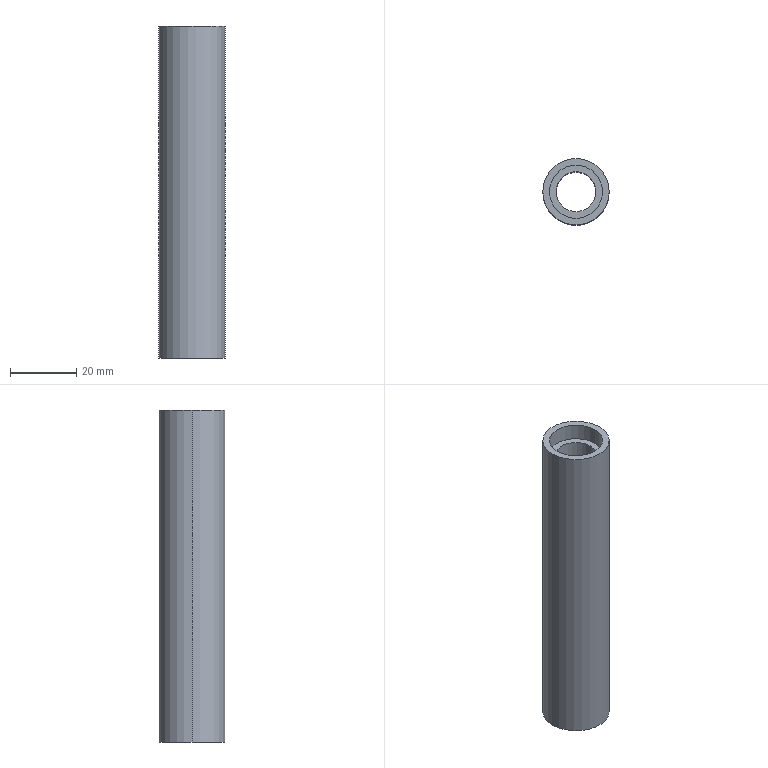Part | STEP file | 11-FG-B06811 | 1 solid | 12 faces | box 20 x 20 x 100 mm | volume 19227 mm3 | cylinder 8 | plane 4 | commonest cylinder face diameters 16 x4 12 x2 20 x2
STEP:
#1=CARTESIAN_POINT('',(-6.,0.,95.));
#2=VERTEX_POINT('',#1);
#3=CARTESIAN_POINT('',(6.,0.,95.));
#4=VERTEX_POINT('',#3);
#5=CARTESIAN_POINT('',(0.,0.,95.));
#6=DIRECTION('',(0.,0.,1.));
#7=DIRECTION('',(1.,0.,0.));
#8=AXIS2_PLACEMENT_3D('',#5,#6,#7);
#9=CIRCLE('',#8,6.);
#10=EDGE_CURVE('',#2,#4,#9,.T.);
#11=ORIENTED_EDGE('',*,*,#10,.T.);
#12=CARTESIAN_POINT('',(6.,0.,5.));
#13=VERTEX_POINT('',#12);
#14=CARTESIAN_POINT('',(6.,0.,100.));
#15=DIRECTION('',(0.,0.,-1.));
#16=VECTOR('',#15,1000.);
#17=LINE('',#14,#16);
#18=EDGE_CURVE('',#4,#13,#17,.T.);
#19=ORIENTED_EDGE('',*,*,#18,.T.);
#20=CARTESIAN_POINT('',(-6.,0.,5.));
#21=VERTEX_POINT('',#20);
#22=CARTESIAN_POINT('',(0.,0.,5.));
#23=DIRECTION('',(0.,0.,-1.));
#24=DIRECTION('',(-1.,0.,0.));
#25=AXIS2_PLACEMENT_3D('',#22,#23,#24);
#26=CIRCLE('',#25,6.);
#27=EDGE_CURVE('',#13,#21,#26,.T.);
#28=ORIENTED_EDGE('',*,*,#27,.T.);
#29=CARTESIAN_POINT('',(-6.,0.,100.));
#30=DIRECTION('',(0.,0.,-1.));
#31=VECTOR('',#30,1000.);
#32=LINE('',#29,#31);
#33=EDGE_CURVE('',#2,#21,#32,.T.);
#34=ORIENTED_EDGE('',*,*,#33,.F.);
#35=EDGE_LOOP('',(#11,#19,#28,#34));
#36=FACE_OUTER_BOUND('',#35,.T.);
#37=CARTESIAN_POINT('',(0.,0.,100.));
#38=DIRECTION('',(0.,0.,-1.));
#39=DIRECTION('',(-1.,0.,0.));
#40=AXIS2_PLACEMENT_3D('',#37,#38,#39);
#41=CYLINDRICAL_SURFACE('',#40,6.);
#42=ADVANCED_FACE('',(#36),#41,.F.);
#43=CARTESIAN_POINT('',(8.,0.,5.));
#44=VERTEX_POINT('',#43);
#45=CARTESIAN_POINT('',(-8.,0.,5.));
#46=VERTEX_POINT('',#45);
#47=CARTESIAN_POINT('',(0.,0.,5.));
#48=DIRECTION('',(0.,0.,-1.));
#49=DIRECTION('',(-1.,0.,0.));
#50=AXIS2_PLACEMENT_3D('',#47,#48,#49);
#51=CIRCLE('',#50,8.);
#52=EDGE_CURVE('',#44,#46,#51,.T.);
#53=ORIENTED_EDGE('',*,*,#52,.F.);
#54=CARTESIAN_POINT('',(8.,0.,0.));
#55=VERTEX_POINT('',#54);
#56=CARTESIAN_POINT('',(8.,0.,5.));
#57=DIRECTION('',(0.,0.,-1.));
#58=VECTOR('',#57,1000.);
#59=LINE('',#56,#58);
#60=EDGE_CURVE('',#44,#55,#59,.T.);
#61=ORIENTED_EDGE('',*,*,#60,.T.);
#62=CARTESIAN_POINT('',(-8.,0.,0.));
#63=VERTEX_POINT('',#62);
#64=CARTESIAN_POINT('',(0.,0.,0.));
#65=DIRECTION('',(0.,0.,-1.));
#66=DIRECTION('',(-1.,0.,0.));
#67=AXIS2_PLACEMENT_3D('',#64,#65,#66);
#68=CIRCLE('',#67,8.);
#69=EDGE_CURVE('',#55,#63,#68,.T.);
#70=ORIENTED_EDGE('',*,*,#69,.T.);
#71=CARTESIAN_POINT('',(-8.,0.,5.));
#72=DIRECTION('',(0.,0.,-1.));
#73=VECTOR('',#72,1000.);
#74=LINE('',#71,#73);
#75=EDGE_CURVE('',#46,#63,#74,.T.);
#76=ORIENTED_EDGE('',*,*,#75,.F.);
#77=EDGE_LOOP('',(#53,#61,#70,#76));
#78=FACE_OUTER_BOUND('',#77,.T.);
#79=CARTESIAN_POINT('',(0.,0.,5.));
#80=DIRECTION('',(0.,0.,-1.));
#81=DIRECTION('',(-1.,0.,0.));
#82=AXIS2_PLACEMENT_3D('',#79,#80,#81);
#83=CYLINDRICAL_SURFACE('',#82,8.);
#84=ADVANCED_FACE('',(#78),#83,.F.);
#85=CARTESIAN_POINT('',(-8.,0.,95.));
#86=VERTEX_POINT('',#85);
#87=CARTESIAN_POINT('',(8.,0.,95.));
#88=VERTEX_POINT('',#87);
#89=CARTESIAN_POINT('',(0.,0.,95.));
#90=DIRECTION('',(0.,0.,1.));
#91=DIRECTION('',(1.,0.,0.));
#92=AXIS2_PLACEMENT_3D('',#89,#90,#91);
#93=CIRCLE('',#92,8.);
#94=EDGE_CURVE('',#86,#88,#93,.T.);
#95=ORIENTED_EDGE('',*,*,#94,.F.);
#96=CARTESIAN_POINT('',(-8.,0.,100.));
#97=VERTEX_POINT('',#96);
#98=CARTESIAN_POINT('',(-8.,0.,95.));
#99=DIRECTION('',(0.,0.,1.));
#100=VECTOR('',#99,1000.);
#101=LINE('',#98,#100);
#102=EDGE_CURVE('',#86,#97,#101,.T.);
#103=ORIENTED_EDGE('',*,*,#102,.T.);
#104=CARTESIAN_POINT('',(8.,0.,100.));
#105=VERTEX_POINT('',#104);
#106=CARTESIAN_POINT('',(0.,0.,100.));
#107=DIRECTION('',(0.,0.,1.));
#108=DIRECTION('',(1.,0.,0.));
#109=AXIS2_PLACEMENT_3D('',#106,#107,#108);
#110=CIRCLE('',#109,8.);
#111=EDGE_CURVE('',#97,#105,#110,.T.);
#112=ORIENTED_EDGE('',*,*,#111,.T.);
#113=CARTESIAN_POINT('',(8.,0.,95.));
#114=DIRECTION('',(0.,0.,1.));
#115=VECTOR('',#114,1000.);
#116=LINE('',#113,#115);
#117=EDGE_CURVE('',#88,#105,#116,.T.);
#118=ORIENTED_EDGE('',*,*,#117,.F.);
#119=EDGE_LOOP('',(#95,#103,#112,#118));
#120=FACE_OUTER_BOUND('',#119,.T.);
#121=CARTESIAN_POINT('',(0.,0.,95.));
#122=DIRECTION('',(0.,0.,1.));
#123=DIRECTION('',(1.,0.,0.));
#124=AXIS2_PLACEMENT_3D('',#121,#122,#123);
#125=CYLINDRICAL_SURFACE('',#124,8.);
#126=ADVANCED_FACE('',(#120),#125,.F.);
#127=CARTESIAN_POINT('',(10.,0.,100.));
#128=VERTEX_POINT('',#127);
#129=CARTESIAN_POINT('',(-10.,0.,100.));
#130=VERTEX_POINT('',#129);
#131=CARTESIAN_POINT('',(0.,0.,100.));
#132=DIRECTION('',(0.,0.,1.));
#133=DIRECTION('',(1.,0.,0.));
#134=AXIS2_PLACEMENT_3D('',#131,#132,#133);
#135=CIRCLE('',#134,10.);
#136=EDGE_CURVE('',#128,#130,#135,.T.);
#137=ORIENTED_EDGE('',*,*,#136,.F.);
#138=CARTESIAN_POINT('',(10.,0.,0.));
#139=VERTEX_POINT('',#138);
#140=CARTESIAN_POINT('',(10.,0.,100.));
#141=DIRECTION('',(0.,0.,-1.));
#142=VECTOR('',#141,1000.);
#143=LINE('',#140,#142);
#144=EDGE_CURVE('',#128,#139,#143,.T.);
#145=ORIENTED_EDGE('',*,*,#144,.T.);
#146=CARTESIAN_POINT('',(-10.,0.,0.));
#147=VERTEX_POINT('',#146);
#148=CARTESIAN_POINT('',(0.,0.,0.));
#149=DIRECTION('',(0.,0.,1.));
#150=DIRECTION('',(1.,0.,0.));
#151=AXIS2_PLACEMENT_3D('',#148,#149,#150);
#152=CIRCLE('',#151,10.);
#153=EDGE_CURVE('',#139,#147,#152,.T.);
#154=ORIENTED_EDGE('',*,*,#153,.T.);
#155=CARTESIAN_POINT('',(-10.,0.,100.));
#156=DIRECTION('',(0.,0.,-1.));
#157=VECTOR('',#156,1000.);
#158=LINE('',#155,#157);
#159=EDGE_CURVE('',#130,#147,#158,.T.);
#160=ORIENTED_EDGE('',*,*,#159,.F.);
#161=EDGE_LOOP('',(#137,#145,#154,#160));
#162=FACE_OUTER_BOUND('',#161,.T.);
#163=CARTESIAN_POINT('',(0.,0.,100.));
#164=DIRECTION('',(0.,0.,-1.));
#165=DIRECTION('',(-1.,0.,0.));
#166=AXIS2_PLACEMENT_3D('',#163,#164,#165);
#167=CYLINDRICAL_SURFACE('',#166,10.);
#168=ADVANCED_FACE('',(#162),#167,.T.);
#169=ORIENTED_EDGE('',*,*,#144,.F.);
#170=CARTESIAN_POINT('',(0.,0.,100.));
#171=DIRECTION('',(0.,0.,1.));
#172=DIRECTION('',(1.,0.,0.));
#173=AXIS2_PLACEMENT_3D('',#170,#171,#172);
#174=CIRCLE('',#173,10.);
#175=EDGE_CURVE('',#130,#128,#174,.T.);
#176=ORIENTED_EDGE('',*,*,#175,.F.);
#177=ORIENTED_EDGE('',*,*,#159,.T.);
#178=CARTESIAN_POINT('',(0.,0.,0.));
#179=DIRECTION('',(0.,0.,1.));
#180=DIRECTION('',(1.,0.,0.));
#181=AXIS2_PLACEMENT_3D('',#178,#179,#180);
#182=CIRCLE('',#181,10.);
#183=EDGE_CURVE('',#147,#139,#182,.T.);
#184=ORIENTED_EDGE('',*,*,#183,.T.);
#185=EDGE_LOOP('',(#169,#176,#177,#184));
#186=FACE_OUTER_BOUND('',#185,.T.);
#187=CARTESIAN_POINT('',(0.,0.,100.));
#188=DIRECTION('',(0.,0.,-1.));
#189=DIRECTION('',(-1.,0.,0.));
#190=AXIS2_PLACEMENT_3D('',#187,#188,#189);
#191=CYLINDRICAL_SURFACE('',#190,10.);
#192=ADVANCED_FACE('',(#186),#191,.T.);
#193=CARTESIAN_POINT('',(0.,0.,100.));
#194=DIRECTION('',(0.,0.,1.));
#195=DIRECTION('',(1.,0.,0.));
#196=AXIS2_PLACEMENT_3D('',#193,#194,#195);
#197=CIRCLE('',#196,8.);
#198=EDGE_CURVE('',#105,#97,#197,.T.);
#199=ORIENTED_EDGE('',*,*,#198,.F.);
#200=ORIENTED_EDGE('',*,*,#111,.F.);
#201=EDGE_LOOP('',(#199,#200));
#202=FACE_BOUND('',#201,.T.);
#203=ORIENTED_EDGE('',*,*,#175,.T.);
#204=ORIENTED_EDGE('',*,*,#136,.T.);
#205=EDGE_LOOP('',(#203,#204));
#206=FACE_OUTER_BOUND('',#205,.T.);
#207=CARTESIAN_POINT('',(0.,0.,100.));
#208=DIRECTION('',(0.,0.,1.));
#209=DIRECTION('',(1.,0.,0.));
#210=AXIS2_PLACEMENT_3D('',#207,#208,#209);
#211=PLANE('',#210);
#212=ADVANCED_FACE('',(#202,#206),#211,.T.);
#213=CARTESIAN_POINT('',(0.,0.,0.));
#214=DIRECTION('',(0.,0.,-1.));
#215=DIRECTION('',(-1.,0.,0.));
#216=AXIS2_PLACEMENT_3D('',#213,#214,#215);
#217=CIRCLE('',#216,8.);
#218=EDGE_CURVE('',#63,#55,#217,.T.);
#219=ORIENTED_EDGE('',*,*,#218,.F.);
#220=ORIENTED_EDGE('',*,*,#69,.F.);
#221=EDGE_LOOP('',(#219,#220));
#222=FACE_BOUND('',#221,.T.);
#223=ORIENTED_EDGE('',*,*,#183,.F.);
#224=ORIENTED_EDGE('',*,*,#153,.F.);
#225=EDGE_LOOP('',(#223,#224));
#226=FACE_OUTER_BOUND('',#225,.T.);
#227=CARTESIAN_POINT('',(0.,0.,0.));
#228=DIRECTION('',(0.,0.,1.));
#229=DIRECTION('',(1.,0.,0.));
#230=AXIS2_PLACEMENT_3D('',#227,#228,#229);
#231=PLANE('',#230);
#232=ADVANCED_FACE('',(#222,#226),#231,.F.);
#233=ORIENTED_EDGE('',*,*,#102,.F.);
#234=CARTESIAN_POINT('',(0.,0.,95.));
#235=DIRECTION('',(0.,0.,1.));
#236=DIRECTION('',(1.,0.,0.));
#237=AXIS2_PLACEMENT_3D('',#234,#235,#236);
#238=CIRCLE('',#237,8.);
#239=EDGE_CURVE('',#88,#86,#238,.T.);
#240=ORIENTED_EDGE('',*,*,#239,.F.);
#241=ORIENTED_EDGE('',*,*,#117,.T.);
#242=ORIENTED_EDGE('',*,*,#198,.T.);
#243=EDGE_LOOP('',(#233,#240,#241,#242));
#244=FACE_OUTER_BOUND('',#243,.T.);
#245=CARTESIAN_POINT('',(0.,0.,95.));
#246=DIRECTION('',(0.,0.,1.));
#247=DIRECTION('',(1.,0.,0.));
#248=AXIS2_PLACEMENT_3D('',#245,#246,#247);
#249=CYLINDRICAL_SURFACE('',#248,8.);
#250=ADVANCED_FACE('',(#244),#249,.F.);
#251=ORIENTED_EDGE('',*,*,#10,.F.);
#252=CARTESIAN_POINT('',(0.,0.,95.));
#253=DIRECTION('',(0.,0.,1.));
#254=DIRECTION('',(1.,0.,0.));
#255=AXIS2_PLACEMENT_3D('',#252,#253,#254);
#256=CIRCLE('',#255,6.);
#257=EDGE_CURVE('',#4,#2,#256,.T.);
#258=ORIENTED_EDGE('',*,*,#257,.F.);
#259=EDGE_LOOP('',(#251,#258));
#260=FACE_BOUND('',#259,.T.);
#261=ORIENTED_EDGE('',*,*,#239,.T.);
#262=ORIENTED_EDGE('',*,*,#94,.T.);
#263=EDGE_LOOP('',(#261,#262));
#264=FACE_OUTER_BOUND('',#263,.T.);
#265=CARTESIAN_POINT('',(0.,0.,95.));
#266=DIRECTION('',(0.,0.,1.));
#267=DIRECTION('',(1.,0.,0.));
#268=AXIS2_PLACEMENT_3D('',#265,#266,#267);
#269=PLANE('',#268);
#270=ADVANCED_FACE('',(#260,#264),#269,.T.);
#271=ORIENTED_EDGE('',*,*,#60,.F.);
#272=CARTESIAN_POINT('',(0.,0.,5.));
#273=DIRECTION('',(0.,0.,-1.));
#274=DIRECTION('',(-1.,0.,0.));
#275=AXIS2_PLACEMENT_3D('',#272,#273,#274);
#276=CIRCLE('',#275,8.);
#277=EDGE_CURVE('',#46,#44,#276,.T.);
#278=ORIENTED_EDGE('',*,*,#277,.F.);
#279=ORIENTED_EDGE('',*,*,#75,.T.);
#280=ORIENTED_EDGE('',*,*,#218,.T.);
#281=EDGE_LOOP('',(#271,#278,#279,#280));
#282=FACE_OUTER_BOUND('',#281,.T.);
#283=CARTESIAN_POINT('',(0.,0.,5.));
#284=DIRECTION('',(0.,0.,-1.));
#285=DIRECTION('',(-1.,0.,0.));
#286=AXIS2_PLACEMENT_3D('',#283,#284,#285);
#287=CYLINDRICAL_SURFACE('',#286,8.);
#288=ADVANCED_FACE('',(#282),#287,.F.);
#289=CARTESIAN_POINT('',(0.,0.,5.));
#290=DIRECTION('',(0.,0.,-1.));
#291=DIRECTION('',(-1.,0.,0.));
#292=AXIS2_PLACEMENT_3D('',#289,#290,#291);
#293=CIRCLE('',#292,6.);
#294=EDGE_CURVE('',#21,#13,#293,.T.);
#295=ORIENTED_EDGE('',*,*,#294,.F.);
#296=ORIENTED_EDGE('',*,*,#27,.F.);
#297=EDGE_LOOP('',(#295,#296));
#298=FACE_BOUND('',#297,.T.);
#299=ORIENTED_EDGE('',*,*,#277,.T.);
#300=ORIENTED_EDGE('',*,*,#52,.T.);
#301=EDGE_LOOP('',(#299,#300));
#302=FACE_OUTER_BOUND('',#301,.T.);
#303=CARTESIAN_POINT('',(0.,0.,5.));
#304=DIRECTION('',(0.,0.,-1.));
#305=DIRECTION('',(-1.,0.,0.));
#306=AXIS2_PLACEMENT_3D('',#303,#304,#305);
#307=PLANE('',#306);
#308=ADVANCED_FACE('',(#298,#302),#307,.T.);
#309=ORIENTED_EDGE('',*,*,#18,.F.);
#310=ORIENTED_EDGE('',*,*,#257,.T.);
#311=ORIENTED_EDGE('',*,*,#33,.T.);
#312=ORIENTED_EDGE('',*,*,#294,.T.);
#313=EDGE_LOOP('',(#309,#310,#311,#312));
#314=FACE_OUTER_BOUND('',#313,.T.);
#315=CARTESIAN_POINT('',(0.,0.,100.));
#316=DIRECTION('',(0.,0.,-1.));
#317=DIRECTION('',(-1.,0.,0.));
#318=AXIS2_PLACEMENT_3D('',#315,#316,#317);
#319=CYLINDRICAL_SURFACE('',#318,6.);
#320=ADVANCED_FACE('',(#314),#319,.F.);
#321=CLOSED_SHELL('',(#42,#84,#126,#168,#192,#212,#232,#250,#270,#288,#308,#320));
#322=MANIFOLD_SOLID_BREP('',#321);
#323=CARTESIAN_POINT('',(0.,0.,0.));
#324=DIRECTION('',(0.,0.,1.));
#325=DIRECTION('',(1.,0.,0.));
#326=AXIS2_PLACEMENT_3D('',#323,#324,#325);
#327=(LENGTH_UNIT()NAMED_UNIT(*)SI_UNIT(.MILLI.,.METRE.));
#328=UNCERTAINTY_MEASURE_WITH_UNIT(LENGTH_MEASURE(0.00001),#327,'','');
#329=(NAMED_UNIT(*)PLANE_ANGLE_UNIT()SI_UNIT($,.RADIAN.));
#330=(NAMED_UNIT(*)SI_UNIT($,.STERADIAN.)SOLID_ANGLE_UNIT());
#331=(GEOMETRIC_REPRESENTATION_CONTEXT(3)GLOBAL_UNCERTAINTY_ASSIGNED_CONTEXT((#328))GLOBAL_UNIT_ASSIGNED_CONTEXT((#327,#329,#330))REPRESENTATION_CONTEXT('',''));
#332=ADVANCED_BREP_SHAPE_REPRESENTATION('',(#322,#326),#331);